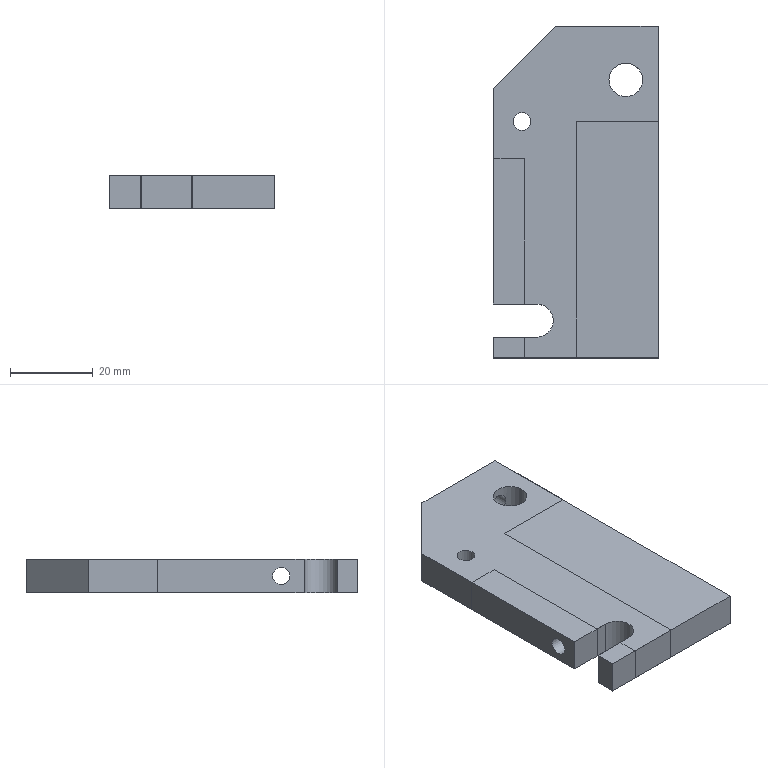NC program | NX | posted with a generic post | part box 40 x 80 x 8 mm
Whole program:
N10 G17 G21 G94 G90
(FLOOR_FACING_COPY_1 , TOOL : D10-30-D10-75-3T-ROUGH)
N12 T01 M6
N14 G54
N16 G17 G0 G90 X2.6 Y-12.1 B0. C0. S3000 M3
N18 G43 Z20. H1
N20 Z2.703 B-180. C-90.
N22 G94 G1 Z-0.297 F1500.
N24 Y-9.1
N26 Y9.1
N28 X9.643
N30 Y-9.1
N32 X16.686
N34 Y9.1
N36 X23.729
N38 Y-9.1
N40 X30.771
N42 Y9.1
N44 X37.814
N46 Y-9.1
N48 X44.857
N50 Y9.1
N52 X51.9
N54 Y-9.1
N56 Y-12.1
N58 Z2.703
N60 G0 Z20.
N62 X2.6
N64 Z2.406
N66 G1 Z-0.594
N68 Y-9.1
N70 Y9.1
N72 X9.643
N74 Y-9.1
N76 X16.686
N78 Y9.1
N80 X23.729
N82 Y-9.1
N84 X30.771
N86 Y9.1
N88 X37.814
N90 Y-9.1
N92 X44.857
N94 Y9.1
N96 X51.9
N98 Y-9.1
N100 Y-12.1
N102 Z2.406
N104 G0 Z20.
N106 X2.6
N108 Z2.109
N110 G1 Z-0.891
N112 Y-9.1
N114 Y9.1
N116 X9.643
N118 Y-9.1
N120 X16.686
N122 Y9.1
N124 X23.729
N126 Y-9.1
N128 X30.771
N130 Y9.1
N132 X37.814
N134 Y-9.1
N136 X44.857
N138 Y9.1
N140 X51.9
N142 Y-9.1
N144 Y-12.1
N146 Z2.109
N148 G0 Z20.
N150 X2.6
N152 Z1.812
N154 G1 Z-1.188
N156 Y-9.1
N158 Y9.1
N160 X9.643
N162 Y-9.1
N164 X16.686
N166 Y9.1
N168 X23.729
N170 Y-9.1
N172 X30.771
N174 Y9.1
N176 X37.814
N178 Y-9.1
N180 X44.857
N182 Y9.1
N184 X51.9
N186 Y-9.1
N188 Y-12.1
N190 Z1.812
N192 G0 Z20.
N194 X2.6
N196 Z1.515
N198 G1 Z-1.485
N200 Y-9.1
N202 Y9.1
N204 X9.643
N206 Y-9.1
N208 X16.686
N210 Y9.1
N212 X23.729
N214 Y-9.1
N216 X30.771
N218 Y9.1
N220 X37.814
N222 Y-9.1
N224 X44.857
N226 Y9.1
N228 X51.9
N230 Y-9.1
N232 Y-12.1
N234 Z1.515
N236 G0 Z20.
N238 X2.6
N240 Z1.218
N242 G1 Z-1.782
N244 Y-9.1
N246 Y9.1
N248 X9.643
N250 Y-9.1
N252 X16.686
N254 Y9.1
N256 X23.729
N258 Y-9.1
N260 X30.771
N262 Y9.1
N264 X37.814
N266 Y-9.1
N268 X44.857
N270 Y9.1
N272 X51.9
N274 Y-9.1
N276 Y-12.1
N278 Z1.218
N280 G0 Z20.
N282 X2.6
N284 Z0.921
N286 G1 Z-2.079
N288 Y-9.1
N290 Y9.1
N292 X9.643
N294 Y-9.1
N296 X16.686
N298 Y9.1
N300 X23.729
N302 Y-9.1
N304 X30.771
N306 Y9.1
N308 X37.814
N310 Y-9.1
N312 X44.857
N314 Y9.1
N316 X51.9
N318 Y-9.1
N320 Y-12.1
N322 Z0.921
N324 G0 Z20.
N326 X2.6
N328 Z0.624
N330 G1 Z-2.376
N332 Y-9.1
N334 Y9.1
N336 X9.643
N338 Y-9.1
N340 X16.686
N342 Y9.1
N344 X23.729
N346 Y-9.1
N348 X30.771
N350 Y9.1
N352 X37.814
N354 Y-9.1
N356 X44.857
N358 Y9.1
N360 X51.9
N362 Y-9.1
N364 Y-12.1
N366 Z0.624
N368 G0 Z20.
N370 X2.6
N372 Z0.327
N374 G1 Z-2.673
N376 Y-9.1
N378 Y9.1
N380 X9.643
N382 Y-9.1
N384 X16.686
N386 Y9.1
N388 X23.729
N390 Y-9.1
N392 X30.771
N394 Y9.1
N396 X37.814
N398 Y-9.1
N400 X44.857
N402 Y9.1
N404 X51.9
N406 Y-9.1
N408 Y-12.1
N410 Z0.327
N412 G0 Z20.
N414 X2.6
N416 Z0.03
N418 G1 Z-2.97
N420 Y-9.1
N422 Y9.1
N424 X9.643
N426 Y-9.1
N428 X16.686
N430 Y9.1
N432 X23.729
N434 Y-9.1
N436 X30.771
N438 Y9.1
N440 X37.814
N442 Y-9.1
N444 X44.857
N446 Y9.1
N448 X51.9
N450 Y-9.1
N452 Y-12.1
N454 Z0.03
N456 G0 Z20.
N458 X2.6
N460 Z-0.267
N462 G1 Z-3.267
N464 Y-9.1
N466 Y9.1
N468 X9.643
N470 Y-9.1
N472 X16.686
N474 Y9.1
N476 X23.729
N478 Y-9.1
N480 X30.771
N482 Y9.1
N484 X37.814
N486 Y-9.1
N488 X44.857
N490 Y9.1
N492 X51.9
N494 Y-9.1
N496 Y-12.1
N498 Z-0.267
N500 G0 Z20.
N502 X2.6
N504 Z-0.564
N506 G1 Z-3.564
N508 Y-9.1
N510 Y9.1
N512 X9.643
N514 Y-9.1
N516 X16.686
N518 Y9.1
N520 X23.729
N522 Y-9.1
N524 X30.771
N526 Y9.1
N528 X37.814
N530 Y-9.1
N532 X44.857
N534 Y9.1
N536 X51.9
N538 Y-9.1
N540 Y-12.1
N542 Z-0.564
N544 G0 Z20.
N546 X2.6
N548 Z-0.861
N550 G1 Z-3.861
N552 Y-9.1
N554 Y9.1
N556 X9.643
N558 Y-9.1
N560 X16.686
N562 Y9.1
N564 X23.729
N566 Y-9.1
N568 X30.771
N570 Y9.1
N572 X37.814
N574 Y-9.1
N576 X44.857
N578 Y9.1
N580 X51.9
N582 Y-9.1
N584 Y-12.1
N586 Z-0.861
N588 G0 Z20.
N590 X2.6
N592 Z-1.158
N594 G1 Z-4.158
N596 Y-9.1
N598 Y9.1
N600 X9.643
N602 Y-9.1
N604 X16.686
N606 Y9.1
N608 X23.729
N610 Y-9.1
N612 X30.771
N614 Y9.1
N616 X37.814
N618 Y-9.1
N620 X44.857
N622 Y9.1
N624 X51.9
N626 Y-9.1
N628 Y-12.1
N630 Z-1.158
N632 G0 Z20.
N634 X2.6
N636 Z-1.455
N638 G1 Z-4.455
N640 Y-9.1
N642 Y9.1
N644 X9.643
N646 Y-9.1
N648 X16.686
N650 Y9.1
N652 X23.729
N654 Y-9.1
N656 X30.771
N658 Y9.1
N660 X37.814
N662 Y-9.1
N664 X44.857
N666 Y9.1
N668 X51.9
N670 Y-9.1
N672 Y-12.1
N674 Z-1.455
N676 G0 Z20.
N678 X2.6
N680 Z-1.752
N682 G1 Z-4.752
N684 Y-9.1
N686 Y9.1
N688 X9.643
N690 Y-9.1
N692 X16.686
N694 Y9.1
N696 X23.729
N698 Y-9.1
N700 X30.771
N702 Y9.1
N704 X37.814
N706 Y-9.1
N708 X44.857
N710 Y9.1
N712 X51.9
N714 Y-9.1
N716 Y-12.1
N718 Z-1.752
N720 G0 Z20.
N722 X2.6
N724 Z-2.049
N726 G1 Z-5.049
N728 Y-9.1
N730 Y9.1
N732 X9.643
N734 Y-9.1
N736 X16.686
N738 Y9.1
N740 X23.729
N742 Y-9.1
N744 X30.771
N746 Y9.1
N748 X37.814
N750 Y-9.1
N752 X44.857
N754 Y9.1
N756 X51.9
N758 Y-9.1
N760 Y-12.1
N762 Z-2.049
N764 G0 Z20.
N766 X2.6
N768 Z-2.346
N770 G1 Z-5.346
N772 Y-9.1
N774 Y9.1
N776 X9.643
N778 Y-9.1
N780 X16.686
N782 Y9.1
N784 X23.729
N786 Y-9.1
N788 X30.771
N790 Y9.1
N792 X37.814
N794 Y-9.1
N796 X44.857
N798 Y9.1
N800 X51.9
N802 Y-9.1
N804 Y-12.1
N806 Z-2.346
N808 G0 Z20.
N810 X2.6
N812 Z-2.643
N814 G1 Z-5.643
N816 Y-9.1
N818 Y9.1
N820 X9.643
N822 Y-9.1
N824 X16.686
N826 Y9.1
N828 X23.729
N830 Y-9.1
N832 X30.771
N834 Y9.1
N836 X37.814
N838 Y-9.1
N840 X44.857
N842 Y9.1
N844 X51.9
N846 Y-9.1
N848 Y-12.1
N850 Z-2.643
N852 G0 Z20.
N854 X2.6
N856 Z-2.94
N858 G1 Z-5.94
N860 Y-9.1
N862 Y9.1
N864 X9.643
N866 Y-9.1
N868 X16.686
N870 Y9.1
N872 X23.729
N874 Y-9.1
N876 X30.771
N878 Y9.1
N880 X37.814
N882 Y-9.1
N884 X44.857
N886 Y9.1
N888 X51.9
N890 Y-9.1
N892 Y-12.1
N894 Z-2.94
N896 G0 Z20.
N898 X2.6
N900 Z-3.237
N902 G1 Z-6.237
N904 Y-9.1
N906 Y9.1
N908 X9.643
N910 Y-9.1
N912 X16.686
N914 Y9.1
N916 X23.729
N918 Y-9.1
N920 X30.771
N922 Y9.1
N924 X37.814
N926 Y-9.1
N928 X44.857
N930 Y9.1
N932 X51.9
N934 Y-9.1
N936 Y-12.1
N938 Z-3.237
N940 G0 Z20.
N942 X2.6
N944 Z-3.534
N946 G1 Z-6.534
N948 Y-9.1
N950 Y9.1
N952 X9.643
N954 Y-9.1
N956 X16.686
N958 Y9.1
N960 X23.729
N962 Y-9.1
N964 X30.771
N966 Y9.1
N968 X37.814
N970 Y-9.1
N972 X44.857
N974 Y9.1
N976 X51.9
N978 Y-9.1
N980 Y-12.1
N982 Z-3.534
N984 G0 Z20.
N986 X2.6
N988 Z-3.831
N990 G1 Z-6.831
N992 Y-9.1
N994 Y9.1
N996 X9.643
N998 Y-9.1
N1000 X16.686
N1002 Y9.1
N1004 X23.729
N1006 Y-9.1
N1008 X30.771
N1010 Y9.1
N1012 X37.814
N1014 Y-9.1
N1016 X44.857
N1018 Y9.1
N1020 X51.9
N1022 Y-9.1
N1024 Y-12.1
N1026 Z-3.831
N1028 G0 Z20.
N1030 X2.6
N1032 Z-4.128
N1034 G1 Z-7.128
N1036 Y-9.1
N1038 Y9.1
N1040 X9.643
N1042 Y-9.1
N1044 X16.686
N1046 Y9.1
N1048 X23.729
N1050 Y-9.1
N1052 X30.771
N1054 Y9.1
N1056 X37.814
N1058 Y-9.1
N1060 X44.857
N1062 Y9.1
N1064 X51.9
N1066 Y-9.1
N1068 Y-12.1
N1070 Z-4.128
N1072 G0 Z20.
N1074 X2.6
N1076 Z-4.425
N1078 G1 Z-7.425
N1080 Y-9.1
N1082 Y9.1
N1084 X9.643
N1086 Y-9.1
N1088 X16.686
N1090 Y9.1
N1092 X23.729
N1094 Y-9.1
N1096 X30.771
N1098 Y9.1
N1100 X37.814
N1102 Y-9.1
N1104 X44.857
N1106 Y9.1
N1108 X51.9
N1110 Y-9.1
N1112 Y-12.1
N1114 Z-4.425
N1116 G0 Z20.
N1118 X2.6
N1120 Z-4.722
N1122 G1 Z-7.722
N1124 Y-9.1
N1126 Y9.1
N1128 X9.643
N1130 Y-9.1
N1132 X16.686
N1134 Y9.1
N1136 X23.729
N1138 Y-9.1
N1140 X30.771
N1142 Y9.1
N1144 X37.814
N1146 Y-9.1
N1148 X44.857
N1150 Y9.1
N1152 X51.9
N1154 Y-9.1
N1156 Y-12.1
N1158 Z-4.722
N1160 G0 Z20.
N1162 X2.6
N1164 Z-5.019
N1166 G1 Z-8.019
N1168 Y-9.1
N1170 Y9.1
N1172 X9.643
N1174 Y-9.1
N1176 X16.686
N1178 Y9.1
N1180 X23.729
N1182 Y-9.1
N1184 X30.771
N1186 Y9.1
N1188 X37.814
N1190 Y-9.1
N1192 X44.857
N1194 Y9.1
N1196 X51.9
N1198 Y-9.1
N1200 Y-12.1
N1202 Z-5.019
N1204 G0 Z20.
N1206 X2.6
N1208 Z-5.316
N1210 G1 Z-8.316
N1212 Y-9.1
N1214 Y9.1
N1216 X9.643
N1218 Y-9.1
N1220 X16.686
N1222 Y9.1
N1224 X23.729
N1226 Y-9.1
N1228 X30.771
N1230 Y9.1
N1232 X37.814
N1234 Y-9.1
N1236 X44.857
N1238 Y9.1
N1240 X51.9
N1242 Y-9.1
N1244 Y-12.1
N1246 Z-5.316
N1248 G0 Z20.
N1250 X2.6
N1252 Z-5.613
N1254 G1 Z-8.613
N1256 Y-9.1
N1258 Y9.1
N1260 X9.643
N1262 Y-9.1
N1264 X16.686
N1266 Y9.1
N1268 X23.729
N1270 Y-9.1
N1272 X30.771
N1274 Y9.1
N1276 X37.814
N1278 Y-9.1
N1280 X44.857
N1282 Y9.1
N1284 X51.9
N1286 Y-9.1
N1288 Y-12.1
N1290 Z-5.613
N1292 G0 Z20.
N1294 X2.6
N1296 Z-5.91
N1298 G1 Z-8.91
N1300 Y-9.1
N1302 Y9.1
N1304 X9.643
N1306 Y-9.1
N1308 X16.686
N1310 Y9.1
N1312 X23.729
N1314 Y-9.1
N1316 X30.771
N1318 Y9.1
N1320 X37.814
N1322 Y-9.1
N1324 X44.857
N1326 Y9.1
N1328 X51.9
N1330 Y-9.1
N1332 Y-12.1
N1334 Z-5.91
N1336 G0 Z20.
N1338 X2.6
N1340 Z-6.207
N1342 G1 Z-9.207
N1344 Y-9.1
N1346 Y9.1
N1348 X9.643
N1350 Y-9.1
N1352 X16.686
N1354 Y9.1
N1356 X23.729
N1358 Y-9.1
N1360 X30.771
N1362 Y9.1
N1364 X37.814
N1366 Y-9.1
N1368 X44.857
N1370 Y9.1
N1372 X51.9
N1374 Y-9.1
N1376 Y-12.1
N1378 Z-6.207
N1380 G0 Z20.
N1382 X2.6
N1384 Z-6.504
N1386 G1 Z-9.504
N1388 Y-9.1
N1390 Y9.1
N1392 X9.643
N1394 Y-9.1
N1396 X16.686
N1398 Y9.1
N1400 X23.729
N1402 Y-9.1
N1404 X30.771
N1406 Y9.1
N1408 X37.814
N1410 Y-9.1
N1412 X44.857
N1414 Y9.1
N1416 X51.9
N1418 Y-9.1
N1420 Y-12.1
N1422 Z-6.504
N1424 G0 Z20.
N1426 X2.6
N1428 Z-6.801
N1430 G1 Z-9.801
N1432 Y-9.1
N1434 Y9.1
N1436 X9.643
N1438 Y-9.1
N1440 X16.686
N1442 Y9.1
N1444 X23.729
N1446 Y-9.1
N1448 X30.771
N1450 Y9.1
N1452 X37.814
N1454 Y-9.1
N1456 X44.857
N1458 Y9.1
N1460 X51.9
N1462 Y-9.1
N1464 Y-12.1
N1466 Z-6.801
N1468 G0 Z20.
N1470 X2.6
N1472 Z-7.099
N1474 G1 Z-10.099
N1476 Y-9.1
N1478 Y9.1
N1480 X9.643
N1482 Y-9.1
N1484 X16.686
N1486 Y9.1
N1488 X23.729
N1490 Y-9.1
N1492 X30.771
N1494 Y9.1
N1496 X37.814
N1498 Y-9.1
N1500 X44.857
N1502 Y9.1
N1504 X51.9
N1506 Y-9.1
N1508 Y-12.1
N1510 Z-7.099
N1512 G0 Z20.
N1514 X2.6
N1516 Z-7.396
N1518 G1 Z-10.396
N1520 Y-9.1
N1522 Y9.1
N1524 X9.643
N1526 Y-9.1
N1528 X16.686
N1530 Y9.1
N1532 X23.729
N1534 Y-9.1
N1536 X30.771
N1538 Y9.1
N1540 X37.814
N1542 Y-9.1
N1544 X44.857
N1546 Y9.1
N1548 X51.9
N1550 Y-9.1
N1552 Y-12.1
N1554 Z-7.396
N1556 G0 Z20.
N1558 X2.6
N1560 Z-7.693
N1562 G1 Z-10.693
N1564 Y-9.1
N1566 Y9.1
N1568 X9.643
N1570 Y-9.1
N1572 X16.686
N1574 Y9.1
N1576 X23.729
N1578 Y-9.1
N1580 X30.771
N1582 Y9.1
N1584 X37.814
N1586 Y-9.1
N1588 X44.857
N1590 Y9.1
N1592 X51.9
N1594 Y-9.1
N1596 Y-12.1
N1598 Z-7.693
N1600 G0 Z20.
N1602 X2.6
N1604 Z-7.99
N1606 G1 Z-10.99
N1608 Y-9.1
N1610 Y9.1
N1612 X9.643
N1614 Y-9.1
N1616 X16.686
N1618 Y9.1
N1620 X23.729
N1622 Y-9.1
N1624 X30.771
N1626 Y9.1
N1628 X37.814
N1630 Y-9.1
N1632 X44.857
N1634 Y9.1
N1636 X51.9
N1638 Y-9.1
N1640 Y-12.1
N1642 Z-7.99
N1644 G0 Z20.
N1646 X2.6
N1648 Z-8.287
N1650 G1 Z-11.287
N1652 Y-9.1
N1654 Y9.1
N1656 X9.643
N1658 Y-9.1
N1660 X16.686
N1662 Y9.1
N1664 X23.729
N1666 Y-9.1
N1668 X30.771
N1670 Y9.1
N1672 X37.814
N1674 Y-9.1
N1676 X44.857
N1678 Y9.1
N1680 X51.9
N1682 Y-9.1
N1684 Y-12.1
N1686 Z-8.287
N1688 G0 Z20.
N1690 X2.6
N1692 Z-8.584
N1694 G1 Z-11.584
N1696 Y-9.1
N1698 Y9.1
N1700 X9.643
N1702 Y-9.1
N1704 X16.686
N1706 Y9.1
N1708 X23.729
N1710 Y-9.1
N1712 X30.771
N1714 Y9.1
N1716 X37.814
N1718 Y-9.1
N1720 X44.857
N1722 Y9.1
N1724 X51.9
N1726 Y-9.1
N1728 Y-12.1
N1730 Z-8.584
N1732 G0 Z20.
N1734 X2.6
N1736 Z-8.881
N1738 G1 Z-11.881
N1740 Y-9.1
N1742 Y9.1
N1744 X9.643
N1746 Y-9.1
N1748 X16.686
N1750 Y9.1
N1752 X23.729
N1754 Y-9.1
N1756 X30.771
N1758 Y9.1
N1760 X37.814
N1762 Y-9.1
N1764 X44.857
N1766 Y9.1
N1768 X51.9
N1770 Y-9.1
N1772 Y-12.1
N1774 Z-8.881
N1776 G0 Z20.
N1778 X2.6
N1780 Z-9.178
N1782 G1 Z-12.178
N1784 Y-9.1
N1786 Y9.1
N1788 X9.643
N1790 Y-9.1
N1792 X16.686
N1794 Y9.1
N1796 X23.729
N1798 Y-9.1
N1800 X30.771
N1802 Y9.1
N1804 X37.814
N1806 Y-9.1
N1808 X44.857
N1810 Y9.1
N1812 X51.9
N1814 Y-9.1
N1816 Y-12.1
N1818 Z-9.178
N1820 G0 Z20.
N1822 X2.6
N1824 Z-9.475
N1826 G1 Z-12.475
N1828 Y-9.1
N1830 Y9.1
N1832 X9.643
N1834 Y-9.1
N1836 X16.686
N1838 Y9.1
N1840 X23.729
N1842 Y-9.1
N1844 X30.771
N1846 Y9.1
N1848 X37.814
N1850 Y-9.1
N1852 X44.857
N1854 Y9.1
N1856 X51.9
N1858 Y-9.1
N1860 Y-12.1
N1862 Z-9.475
N1864 G0 Z20.
N1866 X2.6
N1868 Z-9.772
N1870 G1 Z-12.772
N1872 Y-9.1
N1874 Y9.1
N1876 X9.643
N1878 Y-9.1
N1880 X16.686
N1882 Y9.1
N1884 X23.729
N1886 Y-9.1
N1888 X30.771
N1890 Y9.1
N1892 X37.814
N1894 Y-9.1
N1896 X44.857
N1898 Y9.1
N1900 X51.9
N1902 Y-9.1
N1904 Y-12.1
N1906 Z-9.772
N1908 G0 Z20.
N1910 X2.6
N1912 Z-10.069
N1914 G1 Z-13.069
N1916 Y-9.1
N1918 Y9.1
N1920 X9.643
N1922 Y-9.1
N1924 X16.686
N1926 Y9.1
N1928 X23.729
N1930 Y-9.1
N1932 X30.771
N1934 Y9.1
N1936 X37.814
N1938 Y-9.1
N1940 X44.857
N1942 Y9.1
N1944 X51.9
N1946 Y-9.1
N1948 Y-12.1
N1950 Z-10.069
N1952 G0 Z20.
N1954 X2.6
N1956 Z-10.366
N1958 G1 Z-13.366
N1960 Y-9.1
N1962 Y9.1
N1964 X9.643
N1966 Y-9.1
N1968 X16.686
N1970 Y9.1
N1972 X23.729
N1974 Y-9.1
N1976 X30.771
N1978 Y9.1
N1980 X37.814
N1982 Y-9.1
N1984 X44.857
N1986 Y9.1
N1988 X51.9
N1990 Y-9.1
N1992 Y-12.1
N1994 Z-10.366
N1996 G0 Z20.
N1998 X2.6
N2000 Z-10.663
N2002 G1 Z-13.663
N2004 Y-9.1
N2006 Y9.1
N2008 X9.643
N2010 Y-9.1
N2012 X16.686
N2014 Y9.1
N2016 X23.729
N2018 Y-9.1
N2020 X30.771
N2022 Y9.1
N2024 X37.814
N2026 Y-9.1
N2028 X44.857
N2030 Y9.1
N2032 X51.9
N2034 Y-9.1
N2036 Y-12.1
N2038 Z-10.663
N2040 G0 Z20.
N2042 X2.6
N2044 Z-10.96
N2046 G1 Z-13.96
N2048 Y-9.1
N2050 Y9.1
N2052 X9.643
N2054 Y-9.1
N2056 X16.686
N2058 Y9.1
N2060 X23.729
N2062 Y-9.1
N2064 X30.771
N2066 Y9.1
N2068 X37.814
N2070 Y-9.1
N2072 X44.857
N2074 Y9.1
N2076 X51.9
N2078 Y-9.1
N2080 Y-12.1
N2082 Z-10.96
N2084 G0 Z20.
N2086 X2.6
N2088 Z-11.257
N2090 G1 Z-14.257
N2092 Y-9.1
N2094 Y9.1
N2096 X9.643
N2098 Y-9.1
N2100 X16.686
N2102 Y9.1
N2104 X23.729
N2106 Y-9.1
N2108 X30.771
N2110 Y9.1
N2112 X37.814
N2114 Y-9.1
N2116 X44.857
N2118 Y9.1
N2120 X51.9
N2122 Y-9.1
N2124 Y-12.1
N2126 Z-11.257
N2128 G0 Z20.
N2130 X2.6
N2132 Z-11.554
N2134 G1 Z-14.554
N2136 Y-9.1
N2138 Y9.1
N2140 X9.643
N2142 Y-9.1
N2144 X16.686
N2146 Y9.1
N2148 X23.729
N2150 Y-9.1
N2152 X30.771
N2154 Y9.1
N2156 X37.814
N2158 Y-9.1
N2160 X44.857
N2162 Y9.1
N2164 X51.9
N2166 Y-9.1
N2168 Y-12.1
N2170 Z-11.554
N2172 G0 Z20.
N2174 X2.6
N2176 Z-11.851
N2178 G1 Z-14.851
N2180 Y-9.1
N2182 Y9.1
N2184 X9.643
N2186 Y-9.1
N2188 X16.686
N2190 Y9.1
N2192 X23.729
N2194 Y-9.1
N2196 X30.771
N2198 Y9.1
N2200 X37.814
N2202 Y-9.1
N2204 X44.857
N2206 Y9.1
N2208 X51.9
N2210 Y-9.1
N2212 Y-12.1
N2214 Z-11.851
N2216 G0 Z20.
N2218 X2.6
N2220 Z-12.148
N2222 G1 Z-15.148
N2224 Y-9.1
N2226 Y9.1
N2228 X9.643
N2230 Y-9.1
N2232 X16.686
N2234 Y9.1
N2236 X23.729
N2238 Y-9.1
N2240 X30.771
N2242 Y9.1
N2244 X37.814
N2246 Y-9.1
N2248 X44.857
N2250 Y9.1
N2252 X51.9
N2254 Y-9.1
N2256 Y-12.1
N2258 Z-12.148
N2260 G0 Z20.
N2262 X2.6
N2264 Z-12.445
N2266 G1 Z-15.445
N2268 Y-9.1
N2270 Y9.1
N2272 X9.643
N2274 Y-9.1
N2276 X16.686
N2278 Y9.1
N2280 X23.729
N2282 Y-9.1
N2284 X30.771
N2286 Y9.1
N2288 X37.814
N2290 Y-9.1
N2292 X44.857
N2294 Y9.1
N2296 X51.9
N2298 Y-9.1
N2300 Y-12.1
N2302 Z-12.445
N2304 G0 Z20.
N2306 X2.6
N2308 Z-12.742
N2310 G1 Z-15.742
N2312 Y-9.1
N2314 Y9.1
N2316 X9.643
N2318 Y-9.1
N2320 X16.686
N2322 Y9.1
N2324 X23.729
N2326 Y-9.1
N2328 X30.771
N2330 Y9.1
N2332 X37.814
N2334 Y-9.1
N2336 X44.857
N2338 Y9.1
N2340 X51.9
N2342 Y-9.1
N2344 Y-12.1
N2346 Z-12.742
N2348 G0 Z20.
N2350 X2.6
N2352 Z-13.039
N2354 G1 Z-16.039
N2356 Y-9.1
N2358 Y9.1
N2360 X9.643
N2362 Y-9.1
N2364 X16.686
N2366 Y9.1
N2368 X23.729
N2370 Y-9.1
N2372 X30.771
N2374 Y9.1
N2376 X37.814
N2378 Y-9.1
N2380 X44.857
N2382 Y9.1
N2384 X51.9
N2386 Y-9.1
N2388 Y-12.1
N2390 Z-13.039
N2392 G0 Z20.
N2394 X2.6
N2396 Z-13.336
N2398 G1 Z-16.336
N2400 Y-9.1
N2402 Y9.1
N2404 X9.643
N2406 Y-9.1
N2408 X16.686
N2410 Y9.1
N2412 X23.729
N2414 Y-9.1
N2416 X30.771
N2418 Y9.1
N2420 X37.814
N2422 Y-9.1
N2424 X44.857
N2426 Y9.1
N2428 X51.9
N2430 Y-9.1
N2432 Y-12.1
N2434 Z-13.336
N2436 G0 Z20.
N2438 X2.6
N2440 Z-13.633
N2442 G1 Z-16.633
N2444 Y-9.1
N2446 Y9.1
N2448 X9.643
N2450 Y-9.1
N2452 X16.686
N2454 Y9.1
N2456 X23.729
N2458 Y-9.1
N2460 X30.771
N2462 Y9.1
N2464 X37.814
N2466 Y-9.1
N2468 X44.857
N2470 Y9.1
N2472 X51.9
N2474 Y-9.1
N2476 Y-12.1
N2478 Z-13.633
N2480 G0 Z20.
N2482 X2.6
N2484 Z-13.93
N2486 G1 Z-16.93
N2488 Y-9.1
N2490 Y9.1
N2492 X9.643
N2494 Y-9.1
N2496 X16.686
N2498 Y9.1
N2500 X23.729
N2502 Y-9.1
N2504 X30.771
N2506 Y9.1
N2508 X37.814
N2510 Y-9.1
N2512 X44.857
N2514 Y9.1
N2516 X51.9
N2518 Y-9.1
N2520 Y-12.1
N2522 Z-13.93
N2524 G0 Z20.
N2526 X2.6
N2528 Z-14.227
N2530 G1 Z-17.227
N2532 Y-9.1
N2534 Y9.1
N2536 X9.643
N2538 Y-9.1
N2540 X16.686
N2542 Y9.1
N2544 X23.729
N2546 Y-9.1
N2548 X30.771
N2550 Y9.1
N2552 X37.814
N2554 Y-9.1
N2556 X44.857
N2558 Y9.1
N2560 X51.9
N2562 Y-9.1
N2564 Y-12.1
N2566 Z-14.227
N2568 G0 Z20.
N2570 X2.6
N2572 Z-14.524
N2574 G1 Z-17.524
N2576 Y-9.1
N2578 Y9.1
N2580 X9.643
N2582 Y-9.1
N2584 X16.686
N2586 Y9.1
N2588 X23.729
N2590 Y-9.1
N2592 X30.771
N2594 Y9.1
N2596 X37.814
N2598 Y-9.1
N2600 X44.857
N2602 Y9.1
N2604 X51.9
N2606 Y-9.1
N2608 Y-12.1
N2610 Z-14.524
N2612 G0 Z20.
N2614 X2.6
N2616 Z-14.821
N2618 G1 Z-17.821
N2620 Y-9.1
N2622 Y9.1
N2624 X9.643
N2626 Y-9.1
N2628 X16.686
N2630 Y9.1
N2632 X23.729
N2634 Y-9.1
N2636 X30.771
N2638 Y9.1
N2640 X37.814
N2642 Y-9.1
N2644 X44.857
N2646 Y9.1
N2648 X51.9
N2650 Y-9.1
N2652 Y-12.1
N2654 Z-14.821
N2656 G0 Z20.
N2658 X2.6
N2660 Z-15.118
N2662 G1 Z-18.118
N2664 Y-9.1
N2666 Y9.1
N2668 X9.643
N2670 Y-9.1
N2672 X16.686
N2674 Y9.1
N2676 X23.729
N2678 Y-9.1
N2680 X30.771
N2682 Y9.1
N2684 X37.814
N2686 Y-9.1
N2688 X44.857
N2690 Y9.1
N2692 X51.9
N2694 Y-9.1
N2696 Y-12.1
N2698 Z-15.118
N2700 G0 Z20.
N2702 X2.6
N2704 Z-15.415
N2706 G1 Z-18.415
N2708 Y-9.1
N2710 Y9.1
N2712 X9.643
N2714 Y-9.1
N2716 X16.686
N2718 Y9.1
N2720 X23.729
N2722 Y-9.1
N2724 X30.771
N2726 Y9.1
N2728 X37.814
N2730 Y-9.1
N2732 X44.857
N2734 Y9.1
N2736 X51.9
N2738 Y-9.1
N2740 Y-12.1
N2742 Z-15.415
N2744 G0 Z20.
N2746 X2.6
N2748 Z-15.712
N2750 G1 Z-18.712
N2752 Y-9.1
N2754 Y9.1
N2756 X9.643
N2758 Y-9.1
N2760 X16.686
N2762 Y9.1
N2764 X23.729
N2766 Y-9.1
N2768 X30.771
N2770 Y9.1
N2772 X37.814
N2774 Y-9.1
N2776 X44.857
N2778 Y9.1
N2780 X51.9
N2782 Y-9.1
N2784 Y-12.1
N2786 Z-15.712
N2788 G0 Z20.
N2790 X2.6
N2792 Z-16.009
N2794 G1 Z-19.009
N2796 Y-9.1
N2798 Y9.1
N2800 X9.643
N2802 Y-9.1
N2804 X16.686
N2806 Y9.1
N2808 X23.729
N2810 Y-9.1
N2812 X30.771
N2814 Y9.1
N2816 X37.814
N2818 Y-9.1
N2820 X44.857
N2822 Y9.1
N2824 X51.9
N2826 Y-9.1
N2828 Y-12.1
N2830 Z-16.009
N2832 G0 Z20.
N2834 X2.6
N2836 Z-16.306
N2838 G1 Z-19.306
N2840 Y-9.1
N2842 Y9.1
N2844 X9.643
N2846 Y-9.1
N2848 X16.686
N2850 Y9.1
N2852 X23.729
N2854 Y-9.1
N2856 X30.771
N2858 Y9.1
N2860 X37.814
N2862 Y-9.1
N2864 X44.857
N2866 Y9.1
N2868 X51.9
N2870 Y-9.1
N2872 Y-12.1
N2874 Z-16.306
N2876 G0 Z20.
N2878 X2.6
N2880 Z-16.603
N2882 G1 Z-19.603
N2884 Y-9.1
N2886 Y9.1
N2888 X9.643
N2890 Y-9.1
N2892 X16.686
N2894 Y9.1
N2896 X23.729
N2898 Y-9.1
N2900 X30.771
N2902 Y9.1
N2904 X37.814
N2906 Y-9.1
N2908 X44.857
N2910 Y9.1
N2912 X51.9
N2914 Y-9.1
N2916 Y-12.1
N2918 Z-16.603
N2920 G0 Z20.
N2922 X2.6
N2924 Z-16.9
N2926 G1 Z-19.9
N2928 Y-9.1
N2930 Y9.1
N2932 X9.643
N2934 Y-9.1
N2936 X16.686
N2938 Y9.1
N2940 X23.729
N2942 Y-9.1
N2944 X30.771
N2946 Y9.1
N2948 X37.814
N2950 Y-9.1
N2952 X44.857
N2954 Y9.1
N2956 X51.9
N2958 Y-9.1
N2960 Y-12.1
N2962 Z-16.9
N2964 G0 Z20.
N2966 M5
(PLANAR_MILL_7 , TOOL : 倒角D4-90度)
N2968 T05 M6
N2970 G54
N2972 G17 G0 G90 X55.413 Y-7.992 B0. C0. S3000 M3
N2974 G43 Z20. H5
N2976 Z1.5 B-180. C-90.
N2978 G94 G1 Z-1.5 F800.
N2980 G41 X55.5 Y-7.5 D5
N2982 Y-4.
N2984 Y4.
N2986 Y7.5
N2988 G40
N2990 X55.413 Y7.992
N2992 Z1.5
N2994 G0 Z20.
(PLANAR_MILL_7_COPY , TOOL : 倒角D4-90度)
N2996 X-1.587 Y-7.992
N2998 Z-18.5
N3000 G1 Z-21.5
N3002 G41 X-1.5 Y-7.5
N3004 Y-4.
N3006 Y4.
N3008 Y7.5
N3010 G40
N3012 X-1.587 Y7.992
N3014 Z-18.5
N3016 G0 Z20.
N3018 M5
(DRILLING_3 , TOOL : 倒角D10-90度)
N3020 T02 M6
N3022 G54
N3024 G17 G0 G90 X18.5 Y0. B0. C0. S1200 M3
N3026 G43 Z20. H2
N3028 G94 G81 G99 Z-22.5 B-180. C-90. F60. R-17.
N3030 G80
N3032 G0 X18.5 Y0. Z20.
N3034 M5
(DRILLING_4 , TOOL : 钻头D4.3-54-83)
N3036 T13 M6
N3038 G54
N3040 G17 G0 G90 X18.5 Y0. B0. C0. S1600 M3
N3042 G43 Z20. H13
N3044 G94 G83 G99 Z-36. B-180. C-90. F60. Q2. R-17.
N3046 G80
N3048 G0 X18.5 Y0. Z20.
N3050 M5
(DRILLING_4_COPY , TOOL : 上排M5-22-D5.5-60)
N3052 T12 M6
N3054 G54
N3056 G17 G0 G90 X18.5 Y0. B0. C0. S300 M3
N3058 G43 Z20. H12
N3060 G84 G94 G99 Z-25. B-180. C-90. F240. R-17.
N3062 G80
N3064 G0 X18.5 Y0. Z20.
N3066 M5
(FLOOR_FACING_COPY_1_COPY_COPY , TOOL : D6-18-D6-50-3T-FINISH)
N3068 T06 M6
N3070 G54
N3072 G17 G0 G90 X54. Y-10. B0. C0. S3000 M3
N3074 G43 Z20. H6
N3076 Z-7. B-180. C-90.
N3078 G94 G1 Z-10. F600.
N3080 Y-2.5
N3082 Y2.5
N3084 Y10.
N3086 Z-7.
N3088 G0 Z20.
N3090 Y-10.
N3092 Z-17.
N3094 G1 Z-20.
N3096 Y-2.5
N3098 Y2.5
N3100 Y10.
N3102 Z-17.
N3104 G0 Z20.
(FLOOR_FACING_COPY_1_COPY , TOOL : D6-18-D6-50-3T-FINISH)
N3106 X1.7 Y-10.
N3108 Z-17.
N3110 G1 Z-20.
N3112 Y-7.
N3114 Y7.
N3116 X6.054
N3118 Y-7.
N3120 X10.408
N3122 Y7.
N3124 X14.763
N3126 Y-7.
N3128 X19.117
N3130 Y7.
N3132 X23.471
N3134 Y-7.
N3136 X27.825
N3138 Y7.
N3140 X32.179
N3142 Y-7.
N3144 X36.533
N3146 Y7.
N3148 X40.887
N3150 Y-7.
N3152 X45.242
N3154 Y7.
N3156 X49.596
N3158 Y-7.
N3160 X53.95
N3162 Y7.
N3164 Y10.05
N3166 Z-17.
N3168 G0 Z20.
N3170 M5
N3172 M2